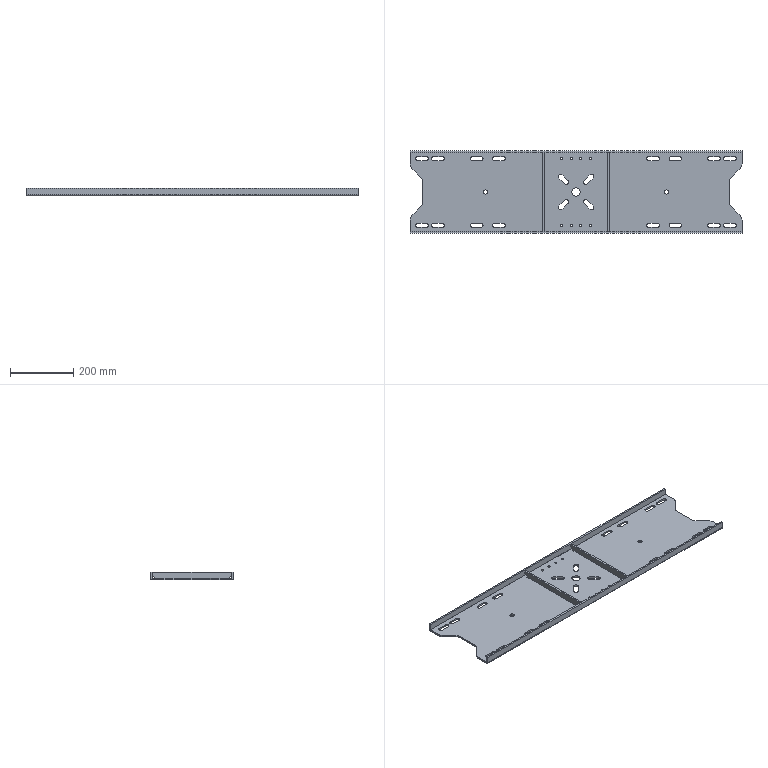Part | 3 solids | 176 faces | box 1046 x 260 x 25 mm | volume 1500679 mm3 | cylinder 94 | plane 82 | commonest cylinder face diameters 13 x52 7 x16 14 x12 40 x8 0.2 x2 10.2 x2